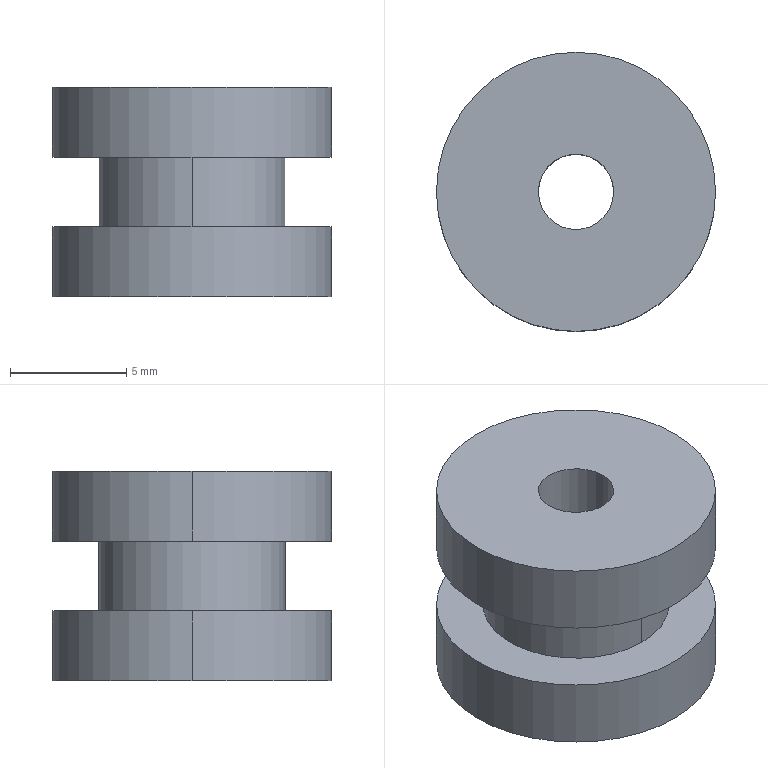Part | SolidWorks | features BaseBody 1 | 1 solid | 12 faces | box 12 x 12 x 9 mm | volume 755.086 mm3 | cylinder 8 | plane 4 | commonest cylinder face diameters 12 x4 3.242 x2 8 x2
STEP:
#1=CARTESIAN_POINT('',(151.613,125.859,6.));
#2=VERTEX_POINT('',#1);
#3=CARTESIAN_POINT('',(139.613,125.859,6.));
#4=VERTEX_POINT('',#3);
#5=CARTESIAN_POINT('',(145.613,125.859,6.));
#6=DIRECTION('',(0.,0.,1.));
#7=DIRECTION('',(1.,0.,0.));
#8=AXIS2_PLACEMENT_3D('',#5,#6,#7);
#9=CIRCLE('',#8,6.);
#10=EDGE_CURVE('',#2,#4,#9,.T.);
#11=ORIENTED_EDGE('',*,*,#10,.T.);
#12=CARTESIAN_POINT('',(139.613,125.859,9.));
#13=VERTEX_POINT('',#12);
#14=CARTESIAN_POINT('',(139.613,125.859,0.));
#15=DIRECTION('',(0.,0.,1.));
#16=VECTOR('',#15,1000.);
#17=LINE('',#14,#16);
#18=EDGE_CURVE('',#4,#13,#17,.T.);
#19=ORIENTED_EDGE('',*,*,#18,.T.);
#20=CARTESIAN_POINT('',(151.613,125.859,9.));
#21=VERTEX_POINT('',#20);
#22=CARTESIAN_POINT('',(145.613,125.859,9.));
#23=DIRECTION('',(0.,0.,-1.));
#24=DIRECTION('',(1.,0.,0.));
#25=AXIS2_PLACEMENT_3D('',#22,#23,#24);
#26=CIRCLE('',#25,6.);
#27=EDGE_CURVE('',#13,#21,#26,.T.);
#28=ORIENTED_EDGE('',*,*,#27,.T.);
#29=CARTESIAN_POINT('',(151.613,125.859,0.));
#30=DIRECTION('',(0.,0.,1.));
#31=VECTOR('',#30,1000.);
#32=LINE('',#29,#31);
#33=EDGE_CURVE('',#2,#21,#32,.T.);
#34=ORIENTED_EDGE('',*,*,#33,.F.);
#35=EDGE_LOOP('',(#11,#19,#28,#34));
#36=FACE_OUTER_BOUND('',#35,.T.);
#37=CARTESIAN_POINT('',(145.613,125.859,0.));
#38=DIRECTION('',(0.,0.,1.));
#39=DIRECTION('',(1.,0.,0.));
#40=AXIS2_PLACEMENT_3D('',#37,#38,#39);
#41=CYLINDRICAL_SURFACE('',#40,6.);
#42=ADVANCED_FACE('',(#36),#41,.T.);
#43=CARTESIAN_POINT('',(145.613,121.859,3.));
#44=VERTEX_POINT('',#43);
#45=CARTESIAN_POINT('',(145.613,129.859,3.));
#46=VERTEX_POINT('',#45);
#47=CARTESIAN_POINT('',(145.613,125.859,3.));
#48=DIRECTION('',(0.,0.,1.));
#49=DIRECTION('',(0.,-1.,0.));
#50=AXIS2_PLACEMENT_3D('',#47,#48,#49);
#51=CIRCLE('',#50,4.);
#52=EDGE_CURVE('',#44,#46,#51,.T.);
#53=ORIENTED_EDGE('',*,*,#52,.T.);
#54=CARTESIAN_POINT('',(145.613,129.859,6.));
#55=VERTEX_POINT('',#54);
#56=CARTESIAN_POINT('',(145.613,129.859,4.5));
#57=DIRECTION('',(0.,0.,1.));
#58=VECTOR('',#57,1000.);
#59=LINE('',#56,#58);
#60=EDGE_CURVE('',#46,#55,#59,.T.);
#61=ORIENTED_EDGE('',*,*,#60,.T.);
#62=CARTESIAN_POINT('',(145.613,121.859,6.));
#63=VERTEX_POINT('',#62);
#64=CARTESIAN_POINT('',(145.613,125.859,6.));
#65=DIRECTION('',(0.,0.,-1.));
#66=DIRECTION('',(0.,-1.,0.));
#67=AXIS2_PLACEMENT_3D('',#64,#65,#66);
#68=CIRCLE('',#67,4.);
#69=EDGE_CURVE('',#55,#63,#68,.T.);
#70=ORIENTED_EDGE('',*,*,#69,.T.);
#71=CARTESIAN_POINT('',(145.613,121.859,4.5));
#72=DIRECTION('',(0.,0.,1.));
#73=VECTOR('',#72,1000.);
#74=LINE('',#71,#73);
#75=EDGE_CURVE('',#44,#63,#74,.T.);
#76=ORIENTED_EDGE('',*,*,#75,.F.);
#77=EDGE_LOOP('',(#53,#61,#70,#76));
#78=FACE_OUTER_BOUND('',#77,.T.);
#79=CARTESIAN_POINT('',(145.613,125.859,4.5));
#80=DIRECTION('',(0.,0.,1.));
#81=DIRECTION('',(0.,-1.,0.));
#82=AXIS2_PLACEMENT_3D('',#79,#80,#81);
#83=CYLINDRICAL_SURFACE('',#82,4.);
#84=ADVANCED_FACE('',(#78),#83,.T.);
#85=CARTESIAN_POINT('',(143.992,125.859,0.));
#86=VERTEX_POINT('',#85);
#87=CARTESIAN_POINT('',(147.234,125.859,0.));
#88=VERTEX_POINT('',#87);
#89=CARTESIAN_POINT('',(145.613,125.859,0.));
#90=DIRECTION('',(0.,0.,1.));
#91=DIRECTION('',(1.,0.,0.));
#92=AXIS2_PLACEMENT_3D('',#89,#90,#91);
#93=CIRCLE('',#92,1.621);
#94=EDGE_CURVE('',#86,#88,#93,.T.);
#95=ORIENTED_EDGE('',*,*,#94,.F.);
#96=CARTESIAN_POINT('',(143.992,125.859,9.));
#97=VERTEX_POINT('',#96);
#98=CARTESIAN_POINT('',(143.992,125.859,-10.209));
#99=DIRECTION('',(0.,0.,1.));
#100=VECTOR('',#99,1000.);
#101=LINE('',#98,#100);
#102=EDGE_CURVE('',#86,#97,#101,.T.);
#103=ORIENTED_EDGE('',*,*,#102,.T.);
#104=CARTESIAN_POINT('',(147.234,125.859,9.));
#105=VERTEX_POINT('',#104);
#106=CARTESIAN_POINT('',(145.613,125.859,9.));
#107=DIRECTION('',(0.,0.,1.));
#108=DIRECTION('',(1.,0.,0.));
#109=AXIS2_PLACEMENT_3D('',#106,#107,#108);
#110=CIRCLE('',#109,1.621);
#111=EDGE_CURVE('',#97,#105,#110,.T.);
#112=ORIENTED_EDGE('',*,*,#111,.T.);
#113=CARTESIAN_POINT('',(147.234,125.859,-10.209));
#114=DIRECTION('',(0.,0.,1.));
#115=VECTOR('',#114,1000.);
#116=LINE('',#113,#115);
#117=EDGE_CURVE('',#88,#105,#116,.T.);
#118=ORIENTED_EDGE('',*,*,#117,.F.);
#119=EDGE_LOOP('',(#95,#103,#112,#118));
#120=FACE_OUTER_BOUND('',#119,.T.);
#121=CARTESIAN_POINT('',(145.613,125.859,-10.209));
#122=DIRECTION('',(0.,0.,1.));
#123=DIRECTION('',(1.,0.,0.));
#124=AXIS2_PLACEMENT_3D('',#121,#122,#123);
#125=CYLINDRICAL_SURFACE('',#124,1.621);
#126=ADVANCED_FACE('',(#120),#125,.F.);
#127=CARTESIAN_POINT('',(139.613,125.859,0.));
#128=VERTEX_POINT('',#127);
#129=CARTESIAN_POINT('',(151.613,125.859,0.));
#130=VERTEX_POINT('',#129);
#131=CARTESIAN_POINT('',(145.613,125.859,0.));
#132=DIRECTION('',(0.,0.,-1.));
#133=DIRECTION('',(1.,0.,0.));
#134=AXIS2_PLACEMENT_3D('',#131,#132,#133);
#135=CIRCLE('',#134,6.);
#136=EDGE_CURVE('',#128,#130,#135,.T.);
#137=ORIENTED_EDGE('',*,*,#136,.F.);
#138=CARTESIAN_POINT('',(139.613,125.859,3.));
#139=VERTEX_POINT('',#138);
#140=CARTESIAN_POINT('',(139.613,125.859,0.));
#141=DIRECTION('',(0.,0.,1.));
#142=VECTOR('',#141,1000.);
#143=LINE('',#140,#142);
#144=EDGE_CURVE('',#128,#139,#143,.T.);
#145=ORIENTED_EDGE('',*,*,#144,.T.);
#146=CARTESIAN_POINT('',(151.613,125.859,3.));
#147=VERTEX_POINT('',#146);
#148=CARTESIAN_POINT('',(145.613,125.859,3.));
#149=DIRECTION('',(0.,0.,-1.));
#150=DIRECTION('',(1.,0.,0.));
#151=AXIS2_PLACEMENT_3D('',#148,#149,#150);
#152=CIRCLE('',#151,6.);
#153=EDGE_CURVE('',#139,#147,#152,.T.);
#154=ORIENTED_EDGE('',*,*,#153,.T.);
#155=CARTESIAN_POINT('',(151.613,125.859,0.));
#156=DIRECTION('',(0.,0.,1.));
#157=VECTOR('',#156,1000.);
#158=LINE('',#155,#157);
#159=EDGE_CURVE('',#130,#147,#158,.T.);
#160=ORIENTED_EDGE('',*,*,#159,.F.);
#161=EDGE_LOOP('',(#137,#145,#154,#160));
#162=FACE_OUTER_BOUND('',#161,.T.);
#163=CARTESIAN_POINT('',(145.613,125.859,0.));
#164=DIRECTION('',(0.,0.,1.));
#165=DIRECTION('',(1.,0.,0.));
#166=AXIS2_PLACEMENT_3D('',#163,#164,#165);
#167=CYLINDRICAL_SURFACE('',#166,6.);
#168=ADVANCED_FACE('',(#162),#167,.T.);
#169=ORIENTED_EDGE('',*,*,#18,.F.);
#170=CARTESIAN_POINT('',(145.613,125.859,6.));
#171=DIRECTION('',(0.,0.,1.));
#172=DIRECTION('',(1.,0.,0.));
#173=AXIS2_PLACEMENT_3D('',#170,#171,#172);
#174=CIRCLE('',#173,6.);
#175=EDGE_CURVE('',#4,#2,#174,.T.);
#176=ORIENTED_EDGE('',*,*,#175,.T.);
#177=ORIENTED_EDGE('',*,*,#33,.T.);
#178=CARTESIAN_POINT('',(145.613,125.859,9.));
#179=DIRECTION('',(0.,0.,-1.));
#180=DIRECTION('',(1.,0.,0.));
#181=AXIS2_PLACEMENT_3D('',#178,#179,#180);
#182=CIRCLE('',#181,6.);
#183=EDGE_CURVE('',#21,#13,#182,.T.);
#184=ORIENTED_EDGE('',*,*,#183,.T.);
#185=EDGE_LOOP('',(#169,#176,#177,#184));
#186=FACE_OUTER_BOUND('',#185,.T.);
#187=CARTESIAN_POINT('',(145.613,125.859,0.));
#188=DIRECTION('',(0.,0.,1.));
#189=DIRECTION('',(1.,0.,0.));
#190=AXIS2_PLACEMENT_3D('',#187,#188,#189);
#191=CYLINDRICAL_SURFACE('',#190,6.);
#192=ADVANCED_FACE('',(#186),#191,.T.);
#193=CARTESIAN_POINT('',(145.613,125.859,6.));
#194=DIRECTION('',(0.,0.,-1.));
#195=DIRECTION('',(0.,-1.,0.));
#196=AXIS2_PLACEMENT_3D('',#193,#194,#195);
#197=CIRCLE('',#196,4.);
#198=EDGE_CURVE('',#63,#55,#197,.T.);
#199=ORIENTED_EDGE('',*,*,#198,.F.);
#200=ORIENTED_EDGE('',*,*,#69,.F.);
#201=EDGE_LOOP('',(#199,#200));
#202=FACE_BOUND('',#201,.T.);
#203=ORIENTED_EDGE('',*,*,#10,.F.);
#204=ORIENTED_EDGE('',*,*,#175,.F.);
#205=EDGE_LOOP('',(#203,#204));
#206=FACE_OUTER_BOUND('',#205,.T.);
#207=CARTESIAN_POINT('',(145.613,130.859,6.));
#208=DIRECTION('',(0.,0.,1.));
#209=DIRECTION('',(1.,0.,0.));
#210=AXIS2_PLACEMENT_3D('',#207,#208,#209);
#211=PLANE('',#210);
#212=ADVANCED_FACE('',(#202,#206),#211,.F.);
#213=CARTESIAN_POINT('',(145.613,125.859,9.));
#214=DIRECTION('',(0.,0.,1.));
#215=DIRECTION('',(1.,0.,0.));
#216=AXIS2_PLACEMENT_3D('',#213,#214,#215);
#217=CIRCLE('',#216,1.621);
#218=EDGE_CURVE('',#105,#97,#217,.T.);
#219=ORIENTED_EDGE('',*,*,#218,.F.);
#220=ORIENTED_EDGE('',*,*,#111,.F.);
#221=EDGE_LOOP('',(#219,#220));
#222=FACE_BOUND('',#221,.T.);
#223=ORIENTED_EDGE('',*,*,#183,.F.);
#224=ORIENTED_EDGE('',*,*,#27,.F.);
#225=EDGE_LOOP('',(#223,#224));
#226=FACE_OUTER_BOUND('',#225,.T.);
#227=CARTESIAN_POINT('',(145.613,125.859,9.));
#228=DIRECTION('',(0.,0.,-1.));
#229=DIRECTION('',(-1.,0.,0.));
#230=AXIS2_PLACEMENT_3D('',#227,#228,#229);
#231=PLANE('',#230);
#232=ADVANCED_FACE('',(#222,#226),#231,.F.);
#233=ORIENTED_EDGE('',*,*,#60,.F.);
#234=CARTESIAN_POINT('',(145.613,125.859,3.));
#235=DIRECTION('',(0.,0.,1.));
#236=DIRECTION('',(0.,-1.,0.));
#237=AXIS2_PLACEMENT_3D('',#234,#235,#236);
#238=CIRCLE('',#237,4.);
#239=EDGE_CURVE('',#46,#44,#238,.T.);
#240=ORIENTED_EDGE('',*,*,#239,.T.);
#241=ORIENTED_EDGE('',*,*,#75,.T.);
#242=ORIENTED_EDGE('',*,*,#198,.T.);
#243=EDGE_LOOP('',(#233,#240,#241,#242));
#244=FACE_OUTER_BOUND('',#243,.T.);
#245=CARTESIAN_POINT('',(145.613,125.859,4.5));
#246=DIRECTION('',(0.,0.,1.));
#247=DIRECTION('',(0.,-1.,0.));
#248=AXIS2_PLACEMENT_3D('',#245,#246,#247);
#249=CYLINDRICAL_SURFACE('',#248,4.);
#250=ADVANCED_FACE('',(#244),#249,.T.);
#251=ORIENTED_EDGE('',*,*,#102,.F.);
#252=CARTESIAN_POINT('',(145.613,125.859,0.));
#253=DIRECTION('',(0.,0.,1.));
#254=DIRECTION('',(1.,0.,0.));
#255=AXIS2_PLACEMENT_3D('',#252,#253,#254);
#256=CIRCLE('',#255,1.621);
#257=EDGE_CURVE('',#88,#86,#256,.T.);
#258=ORIENTED_EDGE('',*,*,#257,.F.);
#259=ORIENTED_EDGE('',*,*,#117,.T.);
#260=ORIENTED_EDGE('',*,*,#218,.T.);
#261=EDGE_LOOP('',(#251,#258,#259,#260));
#262=FACE_OUTER_BOUND('',#261,.T.);
#263=CARTESIAN_POINT('',(145.613,125.859,-10.209));
#264=DIRECTION('',(0.,0.,1.));
#265=DIRECTION('',(1.,0.,0.));
#266=AXIS2_PLACEMENT_3D('',#263,#264,#265);
#267=CYLINDRICAL_SURFACE('',#266,1.621);
#268=ADVANCED_FACE('',(#262),#267,.F.);
#269=ORIENTED_EDGE('',*,*,#52,.F.);
#270=ORIENTED_EDGE('',*,*,#239,.F.);
#271=EDGE_LOOP('',(#269,#270));
#272=FACE_BOUND('',#271,.T.);
#273=CARTESIAN_POINT('',(145.613,125.859,3.));
#274=DIRECTION('',(0.,0.,-1.));
#275=DIRECTION('',(1.,0.,0.));
#276=AXIS2_PLACEMENT_3D('',#273,#274,#275);
#277=CIRCLE('',#276,6.);
#278=EDGE_CURVE('',#147,#139,#277,.T.);
#279=ORIENTED_EDGE('',*,*,#278,.F.);
#280=ORIENTED_EDGE('',*,*,#153,.F.);
#281=EDGE_LOOP('',(#279,#280));
#282=FACE_OUTER_BOUND('',#281,.T.);
#283=CARTESIAN_POINT('',(145.613,130.859,3.));
#284=DIRECTION('',(0.,0.,-1.));
#285=DIRECTION('',(-1.,0.,0.));
#286=AXIS2_PLACEMENT_3D('',#283,#284,#285);
#287=PLANE('',#286);
#288=ADVANCED_FACE('',(#272,#282),#287,.F.);
#289=ORIENTED_EDGE('',*,*,#257,.T.);
#290=ORIENTED_EDGE('',*,*,#94,.T.);
#291=EDGE_LOOP('',(#289,#290));
#292=FACE_BOUND('',#291,.T.);
#293=CARTESIAN_POINT('',(145.613,125.859,0.));
#294=DIRECTION('',(0.,0.,-1.));
#295=DIRECTION('',(1.,0.,0.));
#296=AXIS2_PLACEMENT_3D('',#293,#294,#295);
#297=CIRCLE('',#296,6.);
#298=EDGE_CURVE('',#130,#128,#297,.T.);
#299=ORIENTED_EDGE('',*,*,#298,.T.);
#300=ORIENTED_EDGE('',*,*,#136,.T.);
#301=EDGE_LOOP('',(#299,#300));
#302=FACE_OUTER_BOUND('',#301,.T.);
#303=CARTESIAN_POINT('',(145.613,125.859,0.));
#304=DIRECTION('',(0.,0.,-1.));
#305=DIRECTION('',(-1.,0.,0.));
#306=AXIS2_PLACEMENT_3D('',#303,#304,#305);
#307=PLANE('',#306);
#308=ADVANCED_FACE('',(#292,#302),#307,.T.);
#309=ORIENTED_EDGE('',*,*,#144,.F.);
#310=ORIENTED_EDGE('',*,*,#298,.F.);
#311=ORIENTED_EDGE('',*,*,#159,.T.);
#312=ORIENTED_EDGE('',*,*,#278,.T.);
#313=EDGE_LOOP('',(#309,#310,#311,#312));
#314=FACE_OUTER_BOUND('',#313,.T.);
#315=CARTESIAN_POINT('',(145.613,125.859,0.));
#316=DIRECTION('',(0.,0.,1.));
#317=DIRECTION('',(1.,0.,0.));
#318=AXIS2_PLACEMENT_3D('',#315,#316,#317);
#319=CYLINDRICAL_SURFACE('',#318,6.);
#320=ADVANCED_FACE('',(#314),#319,.T.);
#321=CLOSED_SHELL('',(#42,#84,#126,#168,#192,#212,#232,#250,#268,#288,#308,#320));
#322=MANIFOLD_SOLID_BREP('',#321);
#323=CARTESIAN_POINT('',(0.,0.,0.));
#324=DIRECTION('',(0.,0.,1.));
#325=DIRECTION('',(1.,0.,0.));
#326=AXIS2_PLACEMENT_3D('',#323,#324,#325);
#327=(LENGTH_UNIT()NAMED_UNIT(*)SI_UNIT(.MILLI.,.METRE.));
#328=UNCERTAINTY_MEASURE_WITH_UNIT(LENGTH_MEASURE(0.00001),#327,'','');
#329=(NAMED_UNIT(*)PLANE_ANGLE_UNIT()SI_UNIT($,.RADIAN.));
#330=(NAMED_UNIT(*)SI_UNIT($,.STERADIAN.)SOLID_ANGLE_UNIT());
#331=(GEOMETRIC_REPRESENTATION_CONTEXT(3)GLOBAL_UNCERTAINTY_ASSIGNED_CONTEXT((#328))GLOBAL_UNIT_ASSIGNED_CONTEXT((#327,#329,#330))REPRESENTATION_CONTEXT('',''));
#332=ADVANCED_BREP_SHAPE_REPRESENTATION('',(#322,#326),#331);